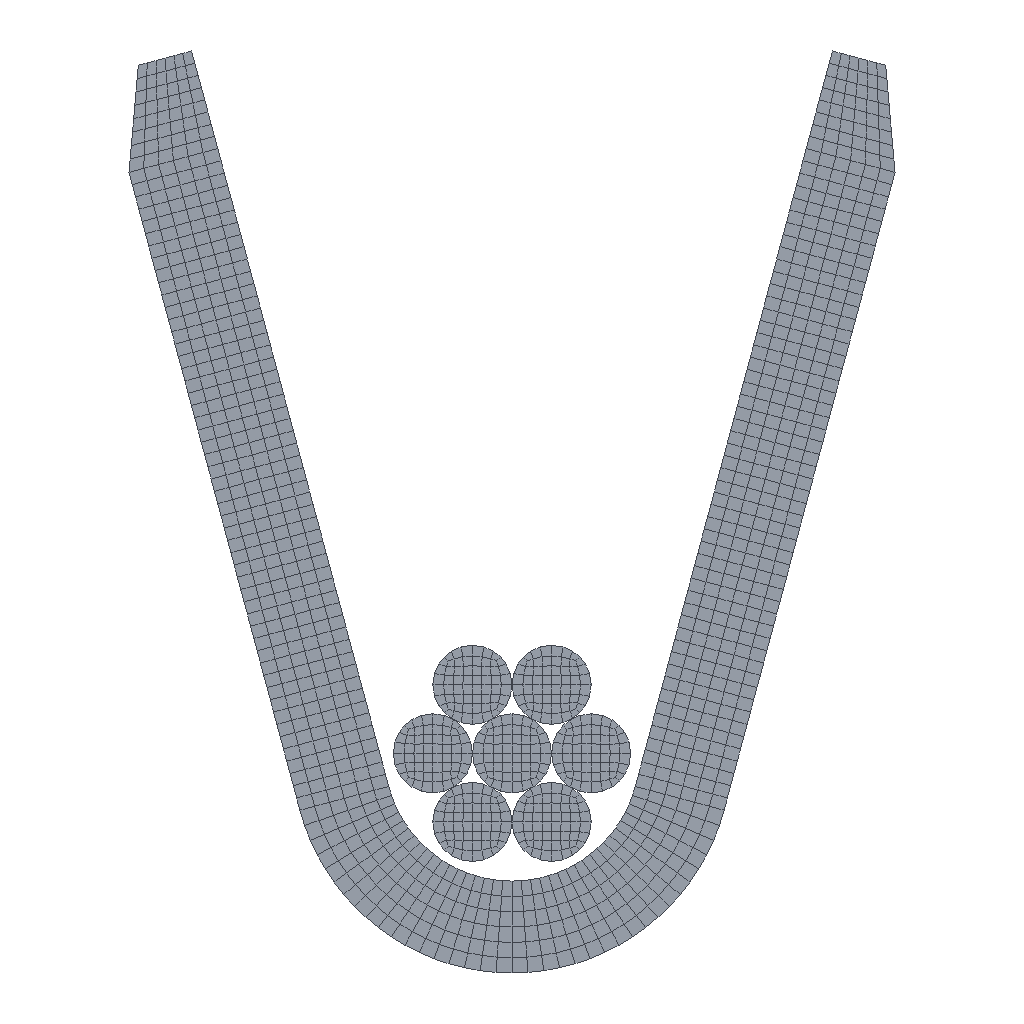Simulation study | abaqus
Set-up summary:
category,name,step,type,value,unit,region
solver,abaqus,,Abaqus/CAE 2024
units,unstated,,unstated,E=17800 density=0.0085 (no match)
analysis,Step-1,,dynamic implicit,nlgeom=True; time_period=0.2
analysis,Step-2,,dynamic implicit,nlgeom=True; time_period=0.01
mesh,nodes,,,1966
mesh,elements,,,1708
element_type,CPS4I,,,936
element_type,CPS4,,,420
element_type,R2D2,,,352
material,copper,,E,17800
material,copper,,nu,0.34
material,copper,,density,0.0085
material,copper,,yield,210
material,copper,,behaviors,plastic; damping
material,grip,,E,100000
material,grip,,nu,0.34
material,grip,,density,0.0085
material,grip,,yield,400
material,grip,,behaviors,plastic; damping
section,grip,,solid section,,,grip
section,copper,,solid section,,,wire
bc,anvil,Step-1,fixed,"[dofs=rz,x,y n=3]",,anvil-1.refPt
bc,punch,Step-1,fixed,"[dofs=rz,x n=2]",,punch-1.refPt
bc,punch,Step-1,displacement,-7.163 [dofs=y],,punch-1.refPt
bc,punch,Step-2,fixed,[dofs=y],,punch-1.refPt
contact,Int-1,initial,general contact,interaction=wire; friction=0.15
constraint,rigid body,,,2
Abaqus input file, long lists of numbers shortened:
**  Plane stress wire crimping analysis
**
**    Model Units are N-mm
**
**    Force   -  Newtons
**    Length  -  Millimeters
**    Time    -  MilliSeconds
**
**    Density -  Grams/mm^3
**
*Heading
** Job name: deck Model name: dynamic
** Generated by: Abaqus/CAE 2024
*Preprint, echo=NO, model=NO, history=NO, contact=NO
**
** PARTS
**
*Part, name=anvil
*Node
      1,  -1.086,  -1.53
      2,  -1.086, -0.7302
** (75 more lines like these left out)
*Element, type=R2D2
 1,  1,  7
 2,  7,  8
** (74 more lines like these left out)
*Node
     78,           0.,         -1.5,           0.
*Nset, nset=anvil-RefPt_, internal
78,
*Nset, nset=refPt
 78,
*Nset, nset=anvil, generate
  1,  77,   1
*Elset, elset=anvil, generate
  1,  76,   1
*Elset, elset=_anvil_SPOS, internal, generate
  1,  76,   1
*Surface, type=ELEMENT, name=anvil
_anvil_SPOS, SPOS
*End Part
**
*Part, name=grip
*Node
      1,   1.152,   2.368
      2,   1.5,   2.275
** (1097 more lines like these left out)
*Element, type=CPS4I
 1,   1,  15, 350,  38
 2,  15,  16, 351, 350
** (934 more lines like these left out)
*Nset, nset=grip, generate
    1,  1099,     1
*Elset, elset=grip, generate
   1,  936,    1
*Elset, elset=_grip_S2, internal, generate
   6,  936,    6
*Elset, elset=_grip_S3, internal
 43, 44, 45, 46, 47, 48, 91, 92, 93, 94, 95, 96
*Elset, elset=_grip_S4, internal, generate
   1,  931,    6
*Surface, type=ELEMENT, name=grip
_grip_S2, S2
_grip_S3, S3
_grip_S4, S4
** Section: grip
*Solid Section, elset=grip, material=grip
1.7,
*End Part
**
*Part, name=punch
*Node
      1,   1.9,      1.816
      2,   1.234,   4.045
** (275 more lines like these left out)
*Element, type=R2D2
 1,  2, 10
 2, 10, 11
** (274 more lines like these left out)
*Node
    278,           0.,           4.,           0.
*Nset, nset=punch-RefPt_, internal
278,
*Nset, nset=refPt
 278,
*Nset, nset=punch, generate
   1,  277,    1
*Elset, elset=punch, generate
   1,  276,    1
*Elset, elset=_punch_SNEG, internal
   1,   2,   3,   4,   5,   6,   7,   8,   9,  10,  11,  12,  13,  14,  15,  16
  17,  18,  19,  20,  21,  22,  23,  24,  25,  26,  27,  28,  29,  30,  31,  32
** (7 more lines like these left out)
*Elset, elset=_punch_SPOS, internal
 108, 109, 110, 111, 112, 113, 114, 115, 116, 117, 118, 119, 120, 121, 122, 123
 124, 125, 126, 127, 128, 129, 130, 131, 132, 133, 134, 135, 136, 137, 138, 170
** (7 more lines like these left out)
*Surface, type=ELEMENT, name=punch
_punch_SNEG, SNEG
_punch_SPOS, SPOS
*End Part
**
*Part, name=wire
*Node
      1,           0.,           0.
      2,           0.,  0.155
** (71 more lines like these left out)
*Element, type=CPS4
 1, 14, 15, 43, 42
 2, 15, 16, 44, 43
** (58 more lines like these left out)
*Nset, nset=wire, generate
  1,  73,   1
*Elset, elset=wire, generate
  1,  60,   1
*Elset, elset=_wire_S2, internal
 10, 11, 12, 28, 29, 30, 43, 44, 45, 55, 56, 57
*Elset, elset=_wire_S1, internal
 13, 14, 15, 16, 17, 18, 31, 32, 33, 58, 59, 60
*Surface, type=ELEMENT, name=wire
_wire_S2, S2
_wire_S1, S1
** Section: wire
*Solid Section, elset=wire, material=copper
2.3,
*End Part
**
**
** ASSEMBLY
**
*Assembly, name=Assembly
**
*Instance, name=grip-1, part=grip
*End Instance
**
*Instance, name=wire-1, part=wire
      -0.155,       0.2685,           0.
*End Instance
**
*Instance, name=wire-2, part=wire
       0.155,       0.2685,           0.
*End Instance
**
*Instance, name=wire-3, part=wire
*End Instance
**
*Instance, name=wire-4, part=wire
0.31,           0.,           0.
*End Instance
**
*Instance, name=wire-5, part=wire
-0.31,           0.,           0.
*End Instance
**
*Instance, name=wire-6, part=wire
-0.155,      -0.2685,           0.
*End Instance
**
*Instance, name=wire-7, part=wire
0.155,      -0.2685,           0.
*End Instance
**
*Instance, name=punch-1, part=punch
*End Instance
**
*Instance, name=anvil-1, part=anvil
*End Instance
**
*Elset, elset=_wires_S2, internal, instance=wire-1
 10, 11, 12, 28, 29, 30, 43, 44, 45, 55, 56, 57
*Elset, elset=_wires_S2, internal, instance=wire-7
 10, 11, 12, 28, 29, 30, 43, 44, 45, 55, 56, 57
*Elset, elset=_wires_S2, internal, instance=wire-2
 10, 11, 12, 28, 29, 30, 43, 44, 45, 55, 56, 57
*Elset, elset=_wires_S2, internal, instance=wire-3
 10, 11, 12, 28, 29, 30, 43, 44, 45, 55, 56, 57
*Elset, elset=_wires_S2, internal, instance=wire-5
 10, 11, 12, 28, 29, 30, 43, 44, 45, 55, 56, 57
*Elset, elset=_wires_S2, internal, instance=wire-4
 10, 11, 12, 28, 29, 30, 43, 44, 45, 55, 56, 57
*Elset, elset=_wires_S2, internal, instance=wire-6
 10, 11, 12, 28, 29, 30, 43, 44, 45, 55, 56, 57
*Elset, elset=_wires_S1, internal, instance=wire-1
 13, 14, 15, 16, 17, 18, 31, 32, 33, 58, 59, 60
*Elset, elset=_wires_S1, internal, instance=wire-7
 13, 14, 15, 16, 17, 18, 31, 32, 33, 58, 59, 60
*Elset, elset=_wires_S1, internal, instance=wire-2
 13, 14, 15, 16, 17, 18, 31, 32, 33, 58, 59, 60
*Elset, elset=_wires_S1, internal, instance=wire-3
 13, 14, 15, 16, 17, 18, 31, 32, 33, 58, 59, 60
*Elset, elset=_wires_S1, internal, instance=wire-5
 13, 14, 15, 16, 17, 18, 31, 32, 33, 58, 59, 60
*Elset, elset=_wires_S1, internal, instance=wire-4
 13, 14, 15, 16, 17, 18, 31, 32, 33, 58, 59, 60
*Elset, elset=_wires_S1, internal, instance=wire-6
 13, 14, 15, 16, 17, 18, 31, 32, 33, 58, 59, 60
*Surface, type=ELEMENT, name=wires
_wires_S2, S2
_wires_S1, S1
** Constraint: anvil
*Rigid Body, ref node=anvil-1.refPt, elset=anvil-1.anvil
** Constraint: punch
*Rigid Body, ref node=punch-1.refPt, elset=punch-1.punch
*Elset, elset=__Int-1_gcs0_16_S2, internal, instance=grip-1, generate
 726,  828,    6
*Surface, type=ELEMENT, name=_Int-1_gcs0_16, internal
__Int-1_gcs0_16_S2, S2
*Elset, elset=__Int-1_gcs0_17_S4, internal, instance=grip-1, generate
 721,  823,    6
*Surface, type=ELEMENT, name=_Int-1_gcs0_17, internal
__Int-1_gcs0_17_S4, S4
*Elset, elset=__Int-1_gcs0_18_S2, internal, instance=grip-1, generate
 834,  936,    6
*Surface, type=ELEMENT, name=_Int-1_gcs0_18, internal
__Int-1_gcs0_18_S2, S2
*Elset, elset=__Int-1_gcs0_19_S4, internal, instance=grip-1, generate
 829,  931,    6
*Surface, type=ELEMENT, name=_Int-1_gcs0_19, internal
__Int-1_gcs0_19_S4, S4
*Elset, elset=__Int-1_gcs0_21_S2, internal, instance=wire-1, generate
 10,  12,   1
*Elset, elset=__Int-1_gcs0_21_S1, internal, instance=wire-1, generate
 13,  15,   1
*Surface, type=ELEMENT, name=_Int-1_gcs0_21, internal
__Int-1_gcs0_21_S2, S2
__Int-1_gcs0_21_S1, S1
*Elset, elset=__Int-1_gcs0_24_S1, internal, instance=wire-1, generate
 16,  18,   1
*Elset, elset=__Int-1_gcs0_24_S2, internal, instance=wire-1, generate
 28,  30,   1
*Surface, type=ELEMENT, name=_Int-1_gcs0_24, internal
__Int-1_gcs0_24_S1, S1
__Int-1_gcs0_24_S2, S2
*Elset, elset=__Int-1_gcs0_26_S1, internal, instance=wire-1, generate
 31,  33,   1
*Elset, elset=__Int-1_gcs0_26_S2, internal, instance=wire-1, generate
 43,  45,   1
*Surface, type=ELEMENT, name=_Int-1_gcs0_26, internal
__Int-1_gcs0_26_S1, S1
__Int-1_gcs0_26_S2, S2
*Elset, elset=__Int-1_gcs0_27_S2, internal, instance=wire-1, generate
 55,  57,   1
*Elset, elset=__Int-1_gcs0_27_S1, internal, instance=wire-1, generate
 58,  60,   1
*Surface, type=ELEMENT, name=_Int-1_gcs0_27, internal
__Int-1_gcs0_27_S2, S2
__Int-1_gcs0_27_S1, S1
*Elset, elset=__Int-1_gcs0_29_S2, internal, instance=wire-2, generate
 10,  12,   1
*Elset, elset=__Int-1_gcs0_29_S1, internal, instance=wire-2, generate
 13,  15,   1
*Surface, type=ELEMENT, name=_Int-1_gcs0_29, internal
__Int-1_gcs0_29_S2, S2
__Int-1_gcs0_29_S1, S1
*Elset, elset=__Int-1_gcs0_32_S1, internal, instance=wire-2, generate
 16,  18,   1
*Elset, elset=__Int-1_gcs0_32_S2, internal, instance=wire-2, generate
 28,  30,   1
*Surface, type=ELEMENT, name=_Int-1_gcs0_32, internal
__Int-1_gcs0_32_S1, S1
__Int-1_gcs0_32_S2, S2
*Elset, elset=__Int-1_gcs0_34_S1, internal, instance=wire-2, generate
 31,  33,   1
*Elset, elset=__Int-1_gcs0_34_S2, internal, instance=wire-2, generate
 43,  45,   1
*Surface, type=ELEMENT, name=_Int-1_gcs0_34, internal
__Int-1_gcs0_34_S1, S1
__Int-1_gcs0_34_S2, S2
*Elset, elset=__Int-1_gcs0_35_S2, internal, instance=wire-2, generate
 55,  57,   1
*Elset, elset=__Int-1_gcs0_35_S1, internal, instance=wire-2, generate
 58,  60,   1
*Surface, type=ELEMENT, name=_Int-1_gcs0_35, internal
__Int-1_gcs0_35_S2, S2
__Int-1_gcs0_35_S1, S1
*Elset, elset=__Int-1_gcs0_37_S2, internal, instance=wire-3, generate
 10,  12,   1
*Elset, elset=__Int-1_gcs0_37_S1, internal, instance=wire-3, generate
 13,  15,   1
*Surface, type=ELEMENT, name=_Int-1_gcs0_37, internal
__Int-1_gcs0_37_S2, S2
__Int-1_gcs0_37_S1, S1
*Elset, elset=__Int-1_gcs0_40_S1, internal, instance=wire-3, generate
 16,  18,   1
*Elset, elset=__Int-1_gcs0_40_S2, internal, instance=wire-3, generate
 28,  30,   1
*Surface, type=ELEMENT, name=_Int-1_gcs0_40, internal
__Int-1_gcs0_40_S1, S1
__Int-1_gcs0_40_S2, S2
*Elset, elset=__Int-1_gcs0_42_S1, internal, instance=wire-3, generate
 31,  33,   1
*Elset, elset=__Int-1_gcs0_42_S2, internal, instance=wire-3, generate
 43,  45,   1
*Surface, type=ELEMENT, name=_Int-1_gcs0_42, internal
__Int-1_gcs0_42_S1, S1
__Int-1_gcs0_42_S2, S2
*Elset, elset=__Int-1_gcs0_43_S2, internal, instance=wire-3, generate
 55,  57,   1
*Elset, elset=__Int-1_gcs0_43_S1, internal, instance=wire-3, generate
 58,  60,   1
*Surface, type=ELEMENT, name=_Int-1_gcs0_43, internal
__Int-1_gcs0_43_S2, S2
__Int-1_gcs0_43_S1, S1
*Elset, elset=__Int-1_gcs0_45_S2, internal, instance=wire-4, generate
 10,  12,   1
*Elset, elset=__Int-1_gcs0_45_S1, internal, instance=wire-4, generate
 13,  15,   1
*Surface, type=ELEMENT, name=_Int-1_gcs0_45, internal
__Int-1_gcs0_45_S2, S2
__Int-1_gcs0_45_S1, S1
*Elset, elset=__Int-1_gcs0_48_S1, internal, instance=wire-4, generate
 16,  18,   1
*Elset, elset=__Int-1_gcs0_48_S2, internal, instance=wire-4, generate
 28,  30,   1
*Surface, type=ELEMENT, name=_Int-1_gcs0_48, internal
__Int-1_gcs0_48_S1, S1
__Int-1_gcs0_48_S2, S2
*Elset, elset=__Int-1_gcs0_50_S1, internal, instance=wire-4, generate
 31,  33,   1
*Elset, elset=__Int-1_gcs0_50_S2, internal, instance=wire-4, generate
 43,  45,   1
*Surface, type=ELEMENT, name=_Int-1_gcs0_50, internal
__Int-1_gcs0_50_S1, S1
__Int-1_gcs0_50_S2, S2
*Elset, elset=__Int-1_gcs0_51_S2, internal, instance=wire-4, generate
 55,  57,   1
*Elset, elset=__Int-1_gcs0_51_S1, internal, instance=wire-4, generate
 58,  60,   1
*Surface, type=ELEMENT, name=_Int-1_gcs0_51, internal
__Int-1_gcs0_51_S2, S2
__Int-1_gcs0_51_S1, S1
*Elset, elset=__Int-1_gcs0_53_S2, internal, instance=wire-5, generate
 10,  12,   1
*Elset, elset=__Int-1_gcs0_53_S1, internal, instance=wire-5, generate
 13,  15,   1
*Surface, type=ELEMENT, name=_Int-1_gcs0_53, internal
__Int-1_gcs0_53_S2, S2
__Int-1_gcs0_53_S1, S1
*Elset, elset=__Int-1_gcs0_56_S1, internal, instance=wire-5, generate
 16,  18,   1
*Elset, elset=__Int-1_gcs0_56_S2, internal, instance=wire-5, generate
 28,  30,   1
*Surface, type=ELEMENT, name=_Int-1_gcs0_56, internal
__Int-1_gcs0_56_S1, S1
__Int-1_gcs0_56_S2, S2
*Elset, elset=__Int-1_gcs0_58_S1, internal, instance=wire-5, generate
 31,  33,   1
*Elset, elset=__Int-1_gcs0_58_S2, internal, instance=wire-5, generate
 43,  45,   1
*Surface, type=ELEMENT, name=_Int-1_gcs0_58, internal
__Int-1_gcs0_58_S1, S1
__Int-1_gcs0_58_S2, S2
*Elset, elset=__Int-1_gcs0_59_S2, internal, instance=wire-5, generate
 55,  57,   1
*Elset, elset=__Int-1_gcs0_59_S1, internal, instance=wire-5, generate
 58,  60,   1
*Surface, type=ELEMENT, name=_Int-1_gcs0_59, internal
__Int-1_gcs0_59_S2, S2
__Int-1_gcs0_59_S1, S1
*Elset, elset=__Int-1_gcs0_61_S2, internal, instance=wire-6, generate
 10,  12,   1
*Elset, elset=__Int-1_gcs0_61_S1, internal, instance=wire-6, generate
 13,  15,   1
*Surface, type=ELEMENT, name=_Int-1_gcs0_61, internal
__Int-1_gcs0_61_S2, S2
__Int-1_gcs0_61_S1, S1
*Elset, elset=__Int-1_gcs0_64_S1, internal, instance=wire-6, generate
 16,  18,   1
*Elset, elset=__Int-1_gcs0_64_S2, internal, instance=wire-6, generate
 28,  30,   1
*Surface, type=ELEMENT, name=_Int-1_gcs0_64, internal
__Int-1_gcs0_64_S1, S1
__Int-1_gcs0_64_S2, S2
*Elset, elset=__Int-1_gcs0_66_S1, internal, instance=wire-6, generate
 31,  33,   1
*Elset, elset=__Int-1_gcs0_66_S2, internal, instance=wire-6, generate
 43,  45,   1
*Surface, type=ELEMENT, name=_Int-1_gcs0_66, internal
__Int-1_gcs0_66_S1, S1
__Int-1_gcs0_66_S2, S2
*Elset, elset=__Int-1_gcs0_67_S2, internal, instance=wire-6, generate
 55,  57,   1
*Elset, elset=__Int-1_gcs0_67_S1, internal, instance=wire-6, generate
 58,  60,   1
*Surface, type=ELEMENT, name=_Int-1_gcs0_67, internal
__Int-1_gcs0_67_S2, S2
__Int-1_gcs0_67_S1, S1
*Elset, elset=__Int-1_gcs0_69_S2, internal, instance=wire-7, generate
 10,  12,   1
*Elset, elset=__Int-1_gcs0_69_S1, internal, instance=wire-7, generate
 13,  15,   1
*Surface, type=ELEMENT, name=_Int-1_gcs0_69, internal
__Int-1_gcs0_69_S2, S2
__Int-1_gcs0_69_S1, S1
*Elset, elset=__Int-1_gcs0_72_S1, internal, instance=wire-7, generate
 16,  18,   1
*Elset, elset=__Int-1_gcs0_72_S2, internal, instance=wire-7, generate
 28,  30,   1
*Surface, type=ELEMENT, name=_Int-1_gcs0_72, internal
__Int-1_gcs0_72_S1, S1
__Int-1_gcs0_72_S2, S2
*Elset, elset=__Int-1_gcs0_74_S1, internal, instance=wire-7, generate
 31,  33,   1
*Elset, elset=__Int-1_gcs0_74_S2, internal, instance=wire-7, generate
 43,  45,   1
*Surface, type=ELEMENT, name=_Int-1_gcs0_74, internal
__Int-1_gcs0_74_S1, S1
__Int-1_gcs0_74_S2, S2
*Elset, elset=__Int-1_gcs0_75_S2, internal, instance=wire-7, generate
 55,  57,   1
*Elset, elset=__Int-1_gcs0_75_S1, internal, instance=wire-7, generate
 58,  60,   1
*Surface, type=ELEMENT, name=_Int-1_gcs0_75, internal
__Int-1_gcs0_75_S2, S2
__Int-1_gcs0_75_S1, S1
*Elset, elset=__Int-1_gcs0_76_SPOS, internal, instance=punch-1, generate
  1,  47,   1
*Surface, type=ELEMENT, name=_Int-1_gcs0_76, internal
__Int-1_gcs0_76_SPOS, SPOS
*Elset, elset=__Int-1_gcs0_78_SPOS, internal, instance=punch-1, generate
 108,  133,    1
*Surface, type=ELEMENT, name=_Int-1_gcs0_78, internal
__Int-1_gcs0_78_SPOS, SPOS
*Elset, elset=__Int-1_gcs0_79_SPOS, internal, instance=punch-1, generate
 134,  138,    1
*Surface, type=ELEMENT, name=_Int-1_gcs0_79, internal
__Int-1_gcs0_79_SPOS, SPOS
*Elset, elset=__Int-1_gcs0_80_SPOS, internal, instance=punch-1, generate
 139,  143,    1
*Surface, type=ELEMENT, name=_Int-1_gcs0_80, internal
__Int-1_gcs0_80_SPOS, SPOS
*Elset, elset=__Int-1_gcs0_81_SPOS, internal, instance=punch-1, generate
 144,  169,    1
*Surface, type=ELEMENT, name=_Int-1_gcs0_81, internal
__Int-1_gcs0_81_SPOS, SPOS
*Elset, elset=__Int-1_gcs0_83_SPOS, internal, instance=punch-1, generate
 230,  276,    1
*Surface, type=ELEMENT, name=_Int-1_gcs0_83, internal
__Int-1_gcs0_83_SPOS, SPOS
*Elset, elset=__Int-1_gcs0_84_SNEG, internal, instance=punch-1, generate
  1,  47,   1
*Surface, type=ELEMENT, name=_Int-1_gcs0_84, internal
__Int-1_gcs0_84_SNEG, SNEG
*Elset, elset=__Int-1_gcs0_86_SNEG, internal, instance=punch-1, generate
 108,  133,    1
*Surface, type=ELEMENT, name=_Int-1_gcs0_86, internal
__Int-1_gcs0_86_SNEG, SNEG
*Elset, elset=__Int-1_gcs0_87_SNEG, internal, instance=punch-1, generate
 134,  138,    1
*Surface, type=ELEMENT, name=_Int-1_gcs0_87, internal
__Int-1_gcs0_87_SNEG, SNEG
*Elset, elset=__Int-1_gcs0_88_SNEG, internal, instance=punch-1, generate
 139,  143,    1
*Surface, type=ELEMENT, name=_Int-1_gcs0_88, internal
__Int-1_gcs0_88_SNEG, SNEG
*Elset, elset=__Int-1_gcs0_89_SNEG, internal, instance=punch-1, generate
 144,  169,    1
*Surface, type=ELEMENT, name=_Int-1_gcs0_89, internal
__Int-1_gcs0_89_SNEG, SNEG
*Elset, elset=__Int-1_gcs0_91_SNEG, internal, instance=punch-1, generate
 230,  276,    1
*Surface, type=ELEMENT, name=_Int-1_gcs0_91, internal
__Int-1_gcs0_91_SNEG, SNEG
*Elset, elset=__Int-1_gcs0_94_SPOS, internal, instance=anvil-1, generate
 21,  56,   1
*Surface, type=ELEMENT, name=_Int-1_gcs0_94, internal
__Int-1_gcs0_94_SPOS, SPOS
*Elset, elset=__Int-1_gcs0_99_SNEG, internal, instance=anvil-1, generate
 21,  56,   1
*Surface, type=ELEMENT, name=_Int-1_gcs0_99, internal
__Int-1_gcs0_99_SNEG, SNEG
*End Assembly
**
** MATERIALS
**
*Material, name=copper
*Damping, beta=0.0002
*Density
 0.0085,
*Elastic
17800., 0.34
*Plastic
  210., 0.
10000.,20.
*Material, name=grip
*Damping, beta=0.0002
*Density
 0.0085,
*Elastic
100000., 0.34
*Plastic
400., 0.
800.,20.
**
** INTERACTION PROPERTIES
**
*Surface Interaction, name=global
1.,
*Friction, slip tolerance=0.005, taumax=300.
 0.15,
*Surface Interaction, name=grip-int
1.,
*Friction, slip tolerance=0.005, taumax=300.
 0.3,
*Surface Interaction, name=gripself
1.,
*Friction
0.,
*Surface Interaction, name=wire
1.,
*Friction, slip tolerance=0.005
 0.15,
**
** INTERACTIONS
**
** Interaction: Int-1
*Contact
*Contact Inclusions, ALL EXTERIOR
*Contact Property Assignment
 ,  , global
grip-1.grip , punch-1.punch , grip-int
grip-1.grip , anvil-1.anvil , grip-int
grip-1.grip ,  , gripself
wires ,  , wire
grip-1.grip , wires , wire
*Surface Property Assignment, property=GEOMETRIC CORRECTION
_Int-1_gcs0_16, Circumferential, 0., 0.
_Int-1_gcs0_17, Circumferential, 0., 0.
_Int-1_gcs0_18, Circumferential, 0., 0.
_Int-1_gcs0_19, Circumferential, 0., 0.
_Int-1_gcs0_21, Circumferential, -0.155, 0.2685
_Int-1_gcs0_24, Circumferential, -0.155, 0.2685
_Int-1_gcs0_26, Circumferential, -0.155, 0.2685
_Int-1_gcs0_27, Circumferential, -0.155, 0.2685
_Int-1_gcs0_29, Circumferential, 0.155, 0.2685
_Int-1_gcs0_32, Circumferential, 0.155, 0.2685
_Int-1_gcs0_34, Circumferential, 0.155, 0.2685
_Int-1_gcs0_35, Circumferential, 0.155, 0.2685
_Int-1_gcs0_37, Circumferential, 0., 0.
_Int-1_gcs0_40, Circumferential, 0., 0.
_Int-1_gcs0_42, Circumferential, 0., 0.
_Int-1_gcs0_43, Circumferential, 0., 0.
_Int-1_gcs0_45, Circumferential, 0.31, 0.
_Int-1_gcs0_48, Circumferential, 0.31, 0.
_Int-1_gcs0_50, Circumferential, 0.31, 0.
_Int-1_gcs0_51, Circumferential, 0.31, 0.
_Int-1_gcs0_53, Circumferential, -0.31, 0.
_Int-1_gcs0_56, Circumferential, -0.31, 0.
_Int-1_gcs0_58, Circumferential, -0.31, 0.
_Int-1_gcs0_59, Circumferential, -0.31, 0.
_Int-1_gcs0_61, Circumferential, -0.155, -0.2685
_Int-1_gcs0_64, Circumferential, -0.155, -0.2685
_Int-1_gcs0_66, Circumferential, -0.155, -0.2685
_Int-1_gcs0_67, Circumferential, -0.155, -0.2685
_Int-1_gcs0_69, Circumferential, 0.155, -0.2685
_Int-1_gcs0_72, Circumferential, 0.155, -0.2685
_Int-1_gcs0_74, Circumferential, 0.155, -0.2685
_Int-1_gcs0_75, Circumferential, 0.155, -0.2685
_Int-1_gcs0_76, Circumferential, 6.226, 4.322
_Int-1_gcs0_78, Circumferential, 0.5296, 6.989
_Int-1_gcs0_79, Circumferential, 4.40448e-16, 7.391
_Int-1_gcs0_80, Circumferential, 4.40448e-16, 7.391
_Int-1_gcs0_81, Circumferential, -0.5296, 6.989
_Int-1_gcs0_83, Circumferential, -6.226, 4.322
_Int-1_gcs0_84, Circumferential, 6.226, 4.322
_Int-1_gcs0_86, Circumferential, 0.5296, 6.989
** (6 more lines like these left out)
** ----------------------------------------------------------------
**
** STEP: Step-1
**
*Step, name=Step-1, nlgeom=YES, inc=1000
*Dynamic,application=QUASI-STATIC,initial=NO
0.01,0.2,2e-06
**
** BOUNDARY CONDITIONS
**
** Name: anvil Type: Displacement/Rotation
*Boundary
anvil-1.refPt, 1, 1
anvil-1.refPt, 2, 2
anvil-1.refPt, 6, 6
** Name: punch Type: Displacement/Rotation
*Boundary
punch-1.refPt, 1, 1
punch-1.refPt, 2, 2, -7.163
punch-1.refPt, 6, 6
**
** OUTPUT REQUESTS
**
*Restart, write, frequency=0
**
** FIELD OUTPUT: F-Output-1
**
*Output, field, variable=PRESELECT, frequency=1
**
** HISTORY OUTPUT: H-Output-2
**
*Output, history, frequency=1
*Energy Output
ALLIE, ALLKE
**
** HISTORY OUTPUT: H-Output-1
**
*Node Output, nset=punch-1.refPt
RF2, U2
*End Step
** ----------------------------------------------------------------
**
** STEP: Step-2
**
*Step, name=Step-2, nlgeom=YES
*Dynamic
0.001,0.01,1e-07
**
** BOUNDARY CONDITIONS
**
** Name: punch Type: Displacement/Rotation
*Boundary
punch-1.refPt, 2, 2
**
** OUTPUT REQUESTS
**
*Restart, write, frequency=0
**
** FIELD OUTPUT: F-Output-1
**
*Output, field, variable=PRESELECT, frequency=1
**
** HISTORY OUTPUT: H-Output-2
**
*Output, history, frequency=1
*Energy Output
ALLIE, ALLKE
**
** HISTORY OUTPUT: H-Output-1
**
*Node Output, nset=punch-1.refPt
RF2, U2
*End Step
Results summary:
result,odb.job_status,,,JOB_STATUS_COMPLETED_SUCCESSFULLY,"consistent, unstated (Abaqus has no unit system)"
result,steps[0].procedure,Step-1,,*DYNAMIC,"consistent, unstated (Abaqus has no unit system)"
result,steps[0].time_period,Step-1,,0.2,"consistent, unstated (Abaqus has no unit system)"
result,steps[0].n_frames,Step-1,,249,"consistent, unstated (Abaqus has no unit system)"
result,steps[0].last_frame.id,Step-1,,248,"consistent, unstated (Abaqus has no unit system)"
result,steps[0].last_frame.value,Step-1,,0.2,"consistent, unstated (Abaqus has no unit system)"
result,steps[0].last_frame.description,Step-1,,Increment    248: Step Time =   0.2,"consistent, unstated (Abaqus has no unit system)"
result,steps[0].completed,Step-1,,True,"consistent, unstated (Abaqus has no unit system)"
result,steps[0].max_U_magnitude,Step-1,,7.163,"consistent, unstated (Abaqus has no unit system)"
result,steps[0].max_S_mises,Step-1,,680.377,"consistent, unstated (Abaqus has no unit system)"
result,steps[0].RF_sum[1],Step-1,,-4.186,"consistent, unstated (Abaqus has no unit system)"
result,steps[0].RF_sum[2],Step-1,,-1.466,"consistent, unstated (Abaqus has no unit system)"
result,steps[1].procedure,Step-2,,*DYNAMIC,"consistent, unstated (Abaqus has no unit system)"
result,steps[1].time_period,Step-2,,0.01,"consistent, unstated (Abaqus has no unit system)"
result,steps[1].n_frames,Step-2,,17,"consistent, unstated (Abaqus has no unit system)"
result,steps[1].last_frame.id,Step-2,,16,"consistent, unstated (Abaqus has no unit system)"
result,steps[1].last_frame.value,Step-2,,0.01,"consistent, unstated (Abaqus has no unit system)"
result,steps[1].last_frame.description,Step-2,,Increment     16: Step Time =   1.0000E-02,"consistent, unstated (Abaqus has no unit system)"
result,steps[1].completed,Step-2,,True,"consistent, unstated (Abaqus has no unit system)"
result,steps[1].max_U_magnitude,Step-2,,3.213,"consistent, unstated (Abaqus has no unit system)"
result,steps[1].max_S_mises,Step-2,,339.213,"consistent, unstated (Abaqus has no unit system)"
result,steps[1].RF_sum[1],Step-2,,0,"consistent, unstated (Abaqus has no unit system)"
result,steps[1].RF_sum[2],Step-2,,0,"consistent, unstated (Abaqus has no unit system)"